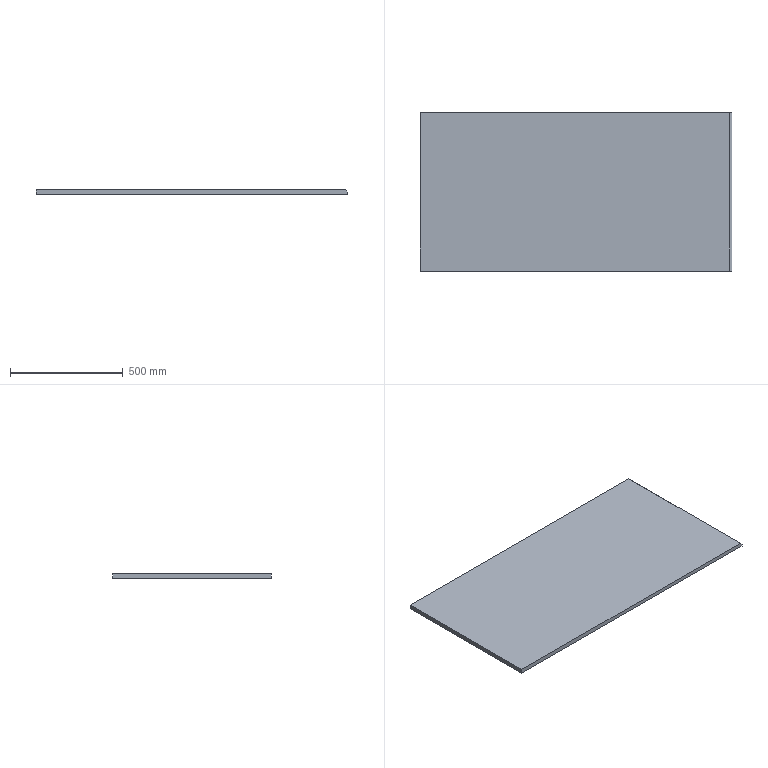Part | SolidWorks | features Chamfer 1, Extrusion 1 | 1 solid | 7 faces | box 1380 x 700 x 20 mm | volume 19285000 mm3 | plane 7
STEP:
#1=CARTESIAN_POINT('',(0.,700.,0.));
#2=VERTEX_POINT('',#1);
#3=CARTESIAN_POINT('',(0.,0.,0.));
#4=VERTEX_POINT('',#3);
#5=CARTESIAN_POINT('',(0.,0.,0.));
#6=DIRECTION('',(0.,-1.,0.));
#7=VECTOR('',#6,1000.);
#8=LINE('',#5,#7);
#9=EDGE_CURVE('',#2,#4,#8,.T.);
#10=ORIENTED_EDGE('',*,*,#9,.T.);
#11=CARTESIAN_POINT('',(0.,0.,20.));
#12=VERTEX_POINT('',#11);
#13=CARTESIAN_POINT('',(0.,0.,20.));
#14=DIRECTION('',(0.,0.,-1.));
#15=VECTOR('',#14,1000.);
#16=LINE('',#13,#15);
#17=EDGE_CURVE('',#12,#4,#16,.T.);
#18=ORIENTED_EDGE('',*,*,#17,.F.);
#19=CARTESIAN_POINT('',(0.,700.,20.));
#20=VERTEX_POINT('',#19);
#21=CARTESIAN_POINT('',(0.,0.,20.));
#22=DIRECTION('',(0.,-1.,0.));
#23=VECTOR('',#22,1000.);
#24=LINE('',#21,#23);
#25=EDGE_CURVE('',#20,#12,#24,.T.);
#26=ORIENTED_EDGE('',*,*,#25,.F.);
#27=CARTESIAN_POINT('',(0.,700.,20.));
#28=DIRECTION('',(0.,0.,-1.));
#29=VECTOR('',#28,1000.);
#30=LINE('',#27,#29);
#31=EDGE_CURVE('',#20,#2,#30,.T.);
#32=ORIENTED_EDGE('',*,*,#31,.T.);
#33=EDGE_LOOP('',(#10,#18,#26,#32));
#34=FACE_OUTER_BOUND('',#33,.T.);
#35=CARTESIAN_POINT('',(0.,0.,20.));
#36=DIRECTION('',(1.,0.,0.));
#37=DIRECTION('',(0.,0.,-1.));
#38=AXIS2_PLACEMENT_3D('',#35,#36,#37);
#39=PLANE('',#38);
#40=ADVANCED_FACE('',(#34),#39,.F.);
#41=CARTESIAN_POINT('',(1380.,0.,10.));
#42=VERTEX_POINT('',#41);
#43=CARTESIAN_POINT('',(1380.,0.,0.));
#44=VERTEX_POINT('',#43);
#45=CARTESIAN_POINT('',(1380.,0.,20.));
#46=DIRECTION('',(0.,0.,-1.));
#47=VECTOR('',#46,1000.);
#48=LINE('',#45,#47);
#49=EDGE_CURVE('',#42,#44,#48,.T.);
#50=ORIENTED_EDGE('',*,*,#49,.F.);
#51=CARTESIAN_POINT('',(1370.,0.,20.));
#52=VERTEX_POINT('',#51);
#53=CARTESIAN_POINT('',(1370.,0.,20.));
#54=DIRECTION('',(-0.7071,0.,0.7071));
#55=VECTOR('',#54,1000.);
#56=LINE('',#53,#55);
#57=EDGE_CURVE('',#42,#52,#56,.T.);
#58=ORIENTED_EDGE('',*,*,#57,.T.);
#59=CARTESIAN_POINT('',(0.,0.,20.));
#60=DIRECTION('',(1.,0.,0.));
#61=VECTOR('',#60,1000.);
#62=LINE('',#59,#61);
#63=EDGE_CURVE('',#12,#52,#62,.T.);
#64=ORIENTED_EDGE('',*,*,#63,.F.);
#65=ORIENTED_EDGE('',*,*,#17,.T.);
#66=CARTESIAN_POINT('',(0.,0.,0.));
#67=DIRECTION('',(1.,0.,0.));
#68=VECTOR('',#67,1000.);
#69=LINE('',#66,#68);
#70=EDGE_CURVE('',#4,#44,#69,.T.);
#71=ORIENTED_EDGE('',*,*,#70,.T.);
#72=EDGE_LOOP('',(#50,#58,#64,#65,#71));
#73=FACE_OUTER_BOUND('',#72,.T.);
#74=CARTESIAN_POINT('',(0.,0.,20.));
#75=DIRECTION('',(0.,1.,0.));
#76=DIRECTION('',(0.,0.,1.));
#77=AXIS2_PLACEMENT_3D('',#74,#75,#76);
#78=PLANE('',#77);
#79=ADVANCED_FACE('',(#73),#78,.F.);
#80=CARTESIAN_POINT('',(1380.,700.,10.));
#81=VERTEX_POINT('',#80);
#82=CARTESIAN_POINT('',(1380.,700.,0.));
#83=VERTEX_POINT('',#82);
#84=CARTESIAN_POINT('',(1380.,700.,20.));
#85=DIRECTION('',(0.,0.,-1.));
#86=VECTOR('',#85,1000.);
#87=LINE('',#84,#86);
#88=EDGE_CURVE('',#81,#83,#87,.T.);
#89=ORIENTED_EDGE('',*,*,#88,.F.);
#90=CARTESIAN_POINT('',(1380.,0.,10.));
#91=DIRECTION('',(0.,-1.,0.));
#92=VECTOR('',#91,1000.);
#93=LINE('',#90,#92);
#94=EDGE_CURVE('',#81,#42,#93,.T.);
#95=ORIENTED_EDGE('',*,*,#94,.T.);
#96=ORIENTED_EDGE('',*,*,#49,.T.);
#97=CARTESIAN_POINT('',(1380.,0.,0.));
#98=DIRECTION('',(0.,1.,0.));
#99=VECTOR('',#98,1000.);
#100=LINE('',#97,#99);
#101=EDGE_CURVE('',#44,#83,#100,.T.);
#102=ORIENTED_EDGE('',*,*,#101,.T.);
#103=EDGE_LOOP('',(#89,#95,#96,#102));
#104=FACE_OUTER_BOUND('',#103,.T.);
#105=CARTESIAN_POINT('',(1380.,0.,20.));
#106=DIRECTION('',(-1.,0.,0.));
#107=DIRECTION('',(0.,0.,1.));
#108=AXIS2_PLACEMENT_3D('',#105,#106,#107);
#109=PLANE('',#108);
#110=ADVANCED_FACE('',(#104),#109,.F.);
#111=CARTESIAN_POINT('',(1370.,700.,20.));
#112=VERTEX_POINT('',#111);
#113=CARTESIAN_POINT('',(0.,700.,20.));
#114=DIRECTION('',(-1.,0.,0.));
#115=VECTOR('',#114,1000.);
#116=LINE('',#113,#115);
#117=EDGE_CURVE('',#112,#20,#116,.T.);
#118=ORIENTED_EDGE('',*,*,#117,.F.);
#119=CARTESIAN_POINT('',(1370.,700.,20.));
#120=DIRECTION('',(0.7071,0.,-0.7071));
#121=VECTOR('',#120,1000.);
#122=LINE('',#119,#121);
#123=EDGE_CURVE('',#112,#81,#122,.T.);
#124=ORIENTED_EDGE('',*,*,#123,.T.);
#125=ORIENTED_EDGE('',*,*,#88,.T.);
#126=CARTESIAN_POINT('',(0.,700.,0.));
#127=DIRECTION('',(-1.,0.,0.));
#128=VECTOR('',#127,1000.);
#129=LINE('',#126,#128);
#130=EDGE_CURVE('',#83,#2,#129,.T.);
#131=ORIENTED_EDGE('',*,*,#130,.T.);
#132=ORIENTED_EDGE('',*,*,#31,.F.);
#133=EDGE_LOOP('',(#118,#124,#125,#131,#132));
#134=FACE_OUTER_BOUND('',#133,.T.);
#135=CARTESIAN_POINT('',(0.,700.,20.));
#136=DIRECTION('',(0.,-1.,0.));
#137=DIRECTION('',(0.,0.,-1.));
#138=AXIS2_PLACEMENT_3D('',#135,#136,#137);
#139=PLANE('',#138);
#140=ADVANCED_FACE('',(#134),#139,.F.);
#141=ORIENTED_EDGE('',*,*,#63,.T.);
#142=CARTESIAN_POINT('',(1370.,0.,20.));
#143=DIRECTION('',(0.,1.,0.));
#144=VECTOR('',#143,1000.);
#145=LINE('',#142,#144);
#146=EDGE_CURVE('',#52,#112,#145,.T.);
#147=ORIENTED_EDGE('',*,*,#146,.T.);
#148=ORIENTED_EDGE('',*,*,#117,.T.);
#149=ORIENTED_EDGE('',*,*,#25,.T.);
#150=EDGE_LOOP('',(#141,#147,#148,#149));
#151=FACE_OUTER_BOUND('',#150,.T.);
#152=CARTESIAN_POINT('',(0.,0.,20.));
#153=DIRECTION('',(0.,0.,-1.));
#154=DIRECTION('',(-1.,0.,0.));
#155=AXIS2_PLACEMENT_3D('',#152,#153,#154);
#156=PLANE('',#155);
#157=ADVANCED_FACE('',(#151),#156,.F.);
#158=ORIENTED_EDGE('',*,*,#9,.F.);
#159=ORIENTED_EDGE('',*,*,#130,.F.);
#160=ORIENTED_EDGE('',*,*,#101,.F.);
#161=ORIENTED_EDGE('',*,*,#70,.F.);
#162=EDGE_LOOP('',(#158,#159,#160,#161));
#163=FACE_OUTER_BOUND('',#162,.T.);
#164=CARTESIAN_POINT('',(0.,0.,0.));
#165=DIRECTION('',(0.,0.,-1.));
#166=DIRECTION('',(-1.,0.,0.));
#167=AXIS2_PLACEMENT_3D('',#164,#165,#166);
#168=PLANE('',#167);
#169=ADVANCED_FACE('',(#163),#168,.T.);
#170=ORIENTED_EDGE('',*,*,#57,.F.);
#171=ORIENTED_EDGE('',*,*,#94,.F.);
#172=ORIENTED_EDGE('',*,*,#123,.F.);
#173=ORIENTED_EDGE('',*,*,#146,.F.);
#174=EDGE_LOOP('',(#170,#171,#172,#173));
#175=FACE_OUTER_BOUND('',#174,.T.);
#176=CARTESIAN_POINT('',(1370.,0.,20.));
#177=DIRECTION('',(-0.7071,0.,-0.7071));
#178=DIRECTION('',(0.,1.,0.));
#179=AXIS2_PLACEMENT_3D('',#176,#177,#178);
#180=PLANE('',#179);
#181=ADVANCED_FACE('',(#175),#180,.F.);
#182=CLOSED_SHELL('',(#40,#79,#110,#140,#157,#169,#181));
#183=MANIFOLD_SOLID_BREP('',#182);
#184=CARTESIAN_POINT('',(0.,0.,0.));
#185=DIRECTION('',(0.,0.,1.));
#186=DIRECTION('',(1.,0.,0.));
#187=AXIS2_PLACEMENT_3D('',#184,#185,#186);
#188=(LENGTH_UNIT()NAMED_UNIT(*)SI_UNIT(.MILLI.,.METRE.));
#189=UNCERTAINTY_MEASURE_WITH_UNIT(LENGTH_MEASURE(0.00001),#188,'','');
#190=(NAMED_UNIT(*)PLANE_ANGLE_UNIT()SI_UNIT($,.RADIAN.));
#191=(NAMED_UNIT(*)SI_UNIT($,.STERADIAN.)SOLID_ANGLE_UNIT());
#192=(GEOMETRIC_REPRESENTATION_CONTEXT(3)GLOBAL_UNCERTAINTY_ASSIGNED_CONTEXT((#189))GLOBAL_UNIT_ASSIGNED_CONTEXT((#188,#190,#191))REPRESENTATION_CONTEXT('',''));
#193=ADVANCED_BREP_SHAPE_REPRESENTATION('',(#183,#187),#192);